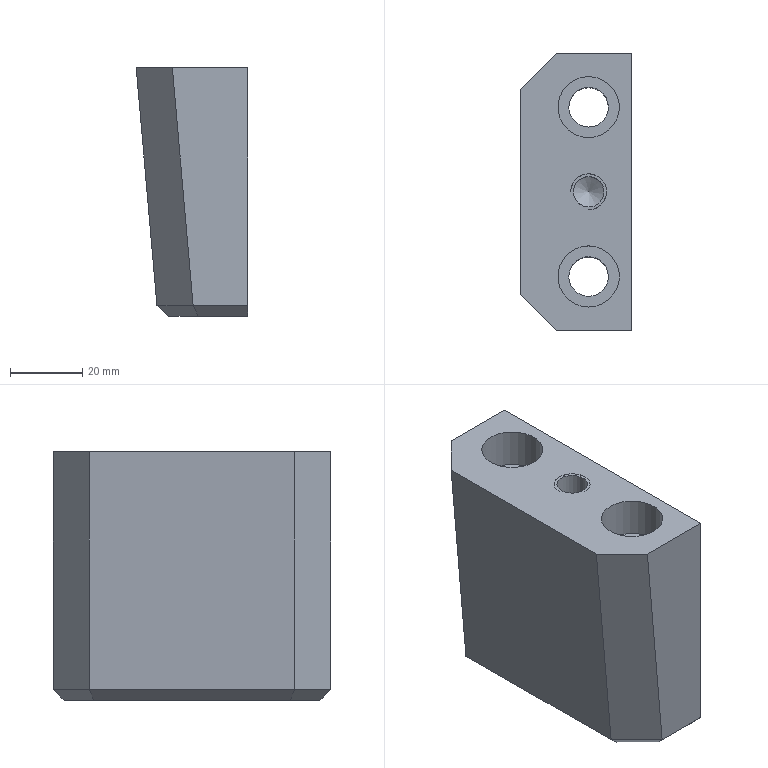Part | STEP file | P011002NM06-000 | 1 solid | 29 faces | box 31 x 77 x 69 mm | volume 123856 mm3 | plane 19 | cylinder 7 | cone 3 | commonest cylinder face diameters 11 x2 17 x2 8.5 x1 9.967 x1 10 x1